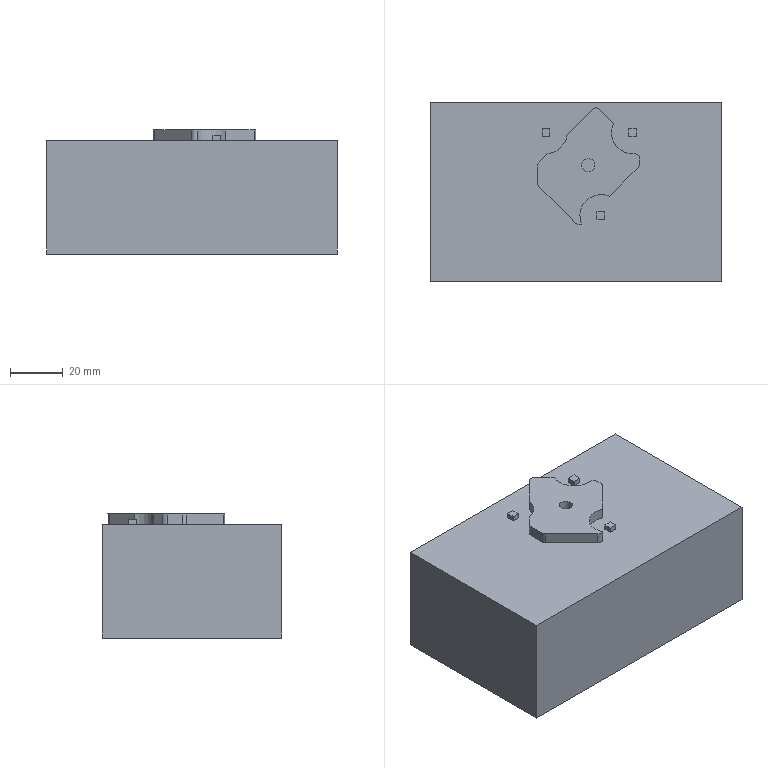NC program | NX | posted with a generic post | part box 110.151 x 68.163 x 47.1 mm
Lines 1467 to 3424 of 32691, first 1659 of 1912 lines:
(CAVITY_MILL_COPY_COPY , TOOL : D10R0)
N2902 T03 M6
N2904 G54
N2906 G17 G0 G90 X-8.338 Y22.938 S5000 M3
N2908 G43 Z80.5 H3
N2910 G94 G1 Z-34. F3000.
N2912 Z-34.5 F1500.
N2914 G3 X-11.214 Y22.865 R188.379
N2916 G1 X-11.344 Y22.861
N2918 G2 X-12.979 Y21.269 R5.579
N2920 G1 X-18.467 Y17.785
N2922 G0 Z-33.8
N2924 X-11.454 Y20.4
N2926 G1 Z-35. F3000.
N2928 X-17.954 F1500.
N2930 X-19.213
N2932 G2 X-20.334 Y20.061 R5.398
N2934 G1 X-26.723 Y18.865
N2936 G0 Z-34.3
N2938 X-11.355 Y20.4
N2940 G1 Z-35.5 F3000.
N2942 X-17.855 F1500.
N2944 X-19.184
N2946 G2 X-20.336 Y20.019 R5.5
N2948 G1 X-26.695 Y18.673
N2950 G0 Z-34.8
N2952 X-11.355 Y20.4
N2954 G1 Z-36. F3000.
N2956 X-17.855 F1500.
N2958 X-19.184
N2960 G2 X-20.336 Y20.019 R5.5
N2962 G1 X-26.695 Y18.673
N2964 G0 Z-35.3
N2966 X-11.355 Y20.4
N2968 G1 Z-36.5 F3000.
N2970 X-17.855 F1500.
N2972 X-19.184
N2974 G2 X-20.336 Y20.019 R5.5
N2976 G1 X-26.695 Y18.673
N2978 G0 Z-35.8
N2980 X-11.355 Y20.4
N2982 G1 Z-37. F3000.
N2984 X-17.855 F1500.
N2986 X-19.184
N2988 G2 X-20.336 Y20.019 R5.5
N2990 G1 X-26.695 Y18.673
N2992 G0 Z80.5
N2994 X-7.629 Y22.95
N2996 G1 Z-34.5 F3000.
N2998 Z-35. F1500.
N3000 G3 X-8.157 Y22.942 R188.379
N3002 X-10.533 Y22.886 R186.972
N3004 G1 X-10.852 Y22.663
N3006 G2 X-12.439 Y21.219 R5.626
N3008 G1 X-17.992 Y17.841
N3010 G0 Z-34.3
N3012 X-6.882 Y22.959
N3014 G1 Z-35. F3000.
N3016 Z-35.5 F1500.
N3018 G3 X-8.157 Y22.942 R188.379
N3020 X-9.727 Y22.908 R186.972
N3022 G1 X-10.131 Y22.663
N3024 X-10.533 Y22.202
N3026 G2 X-11.687 Y21.24 R5.524
N3028 G1 X-17.199 Y17.795
N3030 G0 Z-34.8
N3032 X-6.062 Y22.965
N3034 G1 Z-35.5 F3000.
N3036 Z-36. F1500.
N3038 G3 X-8.913 Y22.927 R189.402
N3040 X-9.594 Y22.347 R2.814
N3042 G2 X-10.824 Y21.273 R5.534
N3044 G1 X-16.298 Y17.769
N3046 G0 Z-35.3
N3048 X-5.086 Y22.968
N3050 G1 Z-36. F3000.
N3052 Z-36.5 F1500.
N3054 G3 X-8.103 Y22.942 R189.402
N3056 G1 X-8.735 Y22.258
N3058 G2 X-9.884 Y21.275 R5.524
N3060 G1 X-15.355 Y17.765
N3062 G0 Z-24.
N3064 X3.06 Y21.256
N3066 G1 Z-34. F3000.
N3068 Z-34.5 F1500.
N3070 G2 X1.548 Y22.663 R5.551
N3072 G1 X0.81 Y22.879
N3074 G3 X-1.65 Y22.939 R185.749
N3076 G0 Z-33.8
N3078 X2.321 Y21.298
N3080 G1 Z-34.5 F3000.
N3082 Z-35. F1500.
N3084 G2 X0.81 Y22.814 R5.053
N3086 G1 X0.018 Y22.902
N3088 G3 X-2.291 Y22.95 R185.749
N3090 G0 Z-34.3
N3092 X1.632 Y21.296
N3094 G1 Z-35. F3000.
N3096 Z-35.5 F1500.
N3098 G2 X0.001 Y22.902 R5.616
N3100 G3 X-2.481 Y22.952 R185.749
N3102 X-3.083 Y22.959 R188.379
N3104 G0 Z-34.8
N3106 X0.859 Y21.287
N3108 G1 Z-35.5 F3000.
N3110 Z-36. F1500.
N3112 G2 X-0.81 Y22.922 R5.664
N3114 G1 X-0.842 Y22.923
N3116 G3 X-3.966 Y22.965 R189.402
N3118 G0 Z-35.3
N3120 X0.008 Y21.244
N3122 G1 Z-36. F3000.
N3124 Z-36.5 F1500.
N3126 G2 X-1.621 Y22.786 R5.593
N3128 G1 X-2.431 Y22.95
N3130 G3 X-2.965 Y22.957 R181.014
N3132 X-4.972 Y22.968 R189.402
N3134 G0 Z-35.8
N3136 X-0.703 Y21.038
N3138 G1 Z-36.5 F3000.
N3140 Z-37. F1500.
N3142 G2 X-2.675 Y22.798 R5.501
N3144 G1 X-3.241 Y22.958
N3146 X-5.645 Y22.967
N3148 X-6.453 Y22.962
N3150 G3 X-7.284 Y22.798 R3.242
N3152 G2 X-9.436 Y20.953 R5.551
N3154 G1 X-15.288 Y18.124
N3156 G0 Z-36.3
N3158 X-6.996 Y13.445
N3160 G1 Z-37.5 F3000.
N3162 X-9.264 Y19.536 F1500.
N3164 X-9.266
N3166 G3 X-13.489 Y14.163 R6.56
N3168 G2 X-14.475 Y13.281 R1.
N3170 G1 Y14.
N3172 G3 X-19.975 Y19.5 R5.5
N3174 G1 X-22.975
N3176 G3 X-28.418 Y14.787 R5.5
N3178 G2 X-29.177 Y15.891 R1.
N3180 G3 X-30.443 Y20.701 R6.56
N3182 G2 X-30.326 Y22.035 R1.
N3184 G3 X-25.975 Y19.9 R5.5
N3186 G1 X-21.475
N3188 G3 X-19.184 Y20.4 R5.5
N3190 G1 X-10.468
N3192 G3 X-8.644 Y20.723 R5.611
N3194 G2 X-9.264 Y19.536 R1.
N3196 G1 X-7.004 Y13.442
N3198 G0 Z-24.
N3200 X-1.466 Y20.78
N3202 G1 Z-37. F3000.
N3204 Z-37.5 F1500.
N3206 G2 X-2.059 Y21.044 R5.797
N3208 X-4.051 Y22.85 R5.402
N3210 G3 X-4.795 Y22.964 R5.482
N3212 G1 X-5.672 Y22.967
N3214 X-5.926 Y22.798
N3216 X-6.121 Y22.528
N3218 G2 X-8.543 Y20.76 R5.611
N3220 G1 X-14.626 Y18.469
N3222 G0 Z-36.8
N3224 X-6.995 Y13.075
N3226 G1 Z-38. F3000.
N3228 X-9.149 Y19.208 F1500.
N3230 G3 X-13.483 Y13.843 R6.56
N3232 G2 X-14.475 Y12.969 R1.
N3234 G1 Y14.
N3236 G3 X-19.975 Y19.5 R5.5
N3238 G1 X-22.975
N3240 G3 X-28.418 Y14.787 R5.5
N3242 G2 X-29.177 Y15.891 R1.
N3244 G3 X-30.443 Y20.701 R6.56
N3246 G2 X-30.326 Y22.035 R1.
N3248 G3 X-25.975 Y19.9 R5.5
N3250 G1 X-21.475
N3252 G3 X-19.184 Y20.4 R5.5
N3254 G1 X-8.783
N3256 X-8.788 Y20.326
N3258 X-8.703 Y20.316
N3260 X-8.691 Y20.389
N3262 G3 X-7.659 Y20.495 R5.482
N3264 G2 X-8.504 Y19.399 R1.002
N3266 G1 X-8.544 Y19.388
N3268 G3 X-9.149 Y19.208 R6.56
N3270 G1 X-6.995 Y13.075
N3272 G0 Z-24.
N3274 X-2.444 Y20.534
N3276 G1 Z-37.5 F3000.
N3278 Z-38. F1500.
N3280 G2 X-4.944 Y21.837 R5.502
N3282 G1 X-5.097 Y21.761
N3284 X-5.264 Y21.624
N3286 G2 X-7.494 Y20.53 R5.482
N3288 G1 X-13.826 Y19.064
N3290 G0 Z-24.
N3292 X0.082 Y14.392
N3294 G1 Z-34.5 F3000.
N3296 X5.683 Y17.69 F1500.
N3298 G3 X3.527 Y19.912 R6.56
N3300 G2 X3.16 Y21.194 R1.
N3302 G3 X5.999 Y20.4 R5.551
N3304 G1 X9.302
N3306 G3 X10.889 Y20.156 R4.677
N3308 G1 X16.023
N3310 G3 X21.082 Y23.438 R5.434
N3312 G2 X21.535 Y22.198 R1.
N3314 G3 X21.552 Y17.401 R6.56
N3316 G2 X21.093 Y16.151 R1.
N3318 G3 X16.048 Y19.5 R5.481
N3320 G1 X13.065
N3322 G3 X7.525 Y14.079 R5.481
N3324 G1 Y13.785
N3326 G2 X6.58 Y14.728 R1.
N3328 G3 X5.683 Y17.69 R6.56
N3330 G1 X0.082 Y14.392
N3332 G0 Z-33.8
N3334 X0.068 Y14.09
N3336 G1 Z-35. F3000.
N3338 X5.54 Y17.599 F1500.
N3340 G3 X3.206 Y19.79 R6.56
N3342 G2 X2.766 Y21.042 R1.
N3344 G3 X5.361 Y20.4 R5.867
N3346 G1 X9.263
N3348 G3 X11.376 Y19.969 R5.124
N3350 G1 X16.025
N3352 G3 X21.13 Y23.415 R5.494
N3354 G2 X21.605 Y22.159 R1.
N3356 G3 X21.623 Y17.302 R6.56
N3358 G2 X21.145 Y16.035 R1.
N3360 G3 X16.048 Y19.5 R5.468
N3362 G1 X13.065
N3364 G3 X7.525 Y14.079 R5.474
N3366 G1 Y13.634
N3368 G2 X6.562 Y14.55 R1.
N3370 G3 X6.522 Y14.911 R6.56
N3372 X5.54 Y17.599 R6.56
N3374 G1 X0.068 Y14.09
N3376 G0 Z-34.3
N3378 X0.074 Y13.794
N3380 G1 Z-35.5 F3000.
N3382 X5.409 Y17.508 F1500.
N3384 G3 X2.876 Y19.668 R6.56
N3386 G2 X2.366 Y20.896 R1.
N3388 G3 X4.648 Y20.4 R5.616
N3390 G1 X9.234
N3392 G3 X11.525 Y19.9 R5.5
N3394 G1 X16.025
N3396 G3 X21.128 Y23.348 R5.5
N3398 G2 X21.605 Y22.096 R1.
N3400 G3 X21.626 Y17.295 R6.56
N3402 G2 X21.147 Y16.031 R1.
N3404 G3 X16.074 Y19.5 R5.468
N3406 G1 X13.065
N3408 G3 X7.525 Y14.079 R5.467
N3410 G1 Y13.523
N3412 G2 X6.552 Y14.421 R1.
N3414 G3 X5.409 Y17.508 R6.56
N3416 G1 X0.074 Y13.794
N3418 G0 Z-34.8
N3420 X0.073 Y13.509
N3422 G1 Z-36. F3000.
N3424 X5.275 Y17.407 F1500.
N3426 G3 X2.419 Y19.58 R6.56
N3428 G2 X1.825 Y20.795 R1.
N3430 G3 X3.847 Y20.4 R5.664
N3432 G1 X9.234
N3434 G3 X11.525 Y19.9 R5.5
N3436 G1 X16.025
N3438 G3 X21.124 Y23.338 R5.5
N3440 G2 X21.598 Y22.085 R1.
N3442 G3 X21.579 Y17.364 R6.56
N3444 G2 X21.11 Y16.123 R1.
N3446 G3 X16.025 Y19.5 R5.468
N3448 G1 X13.065
N3450 G3 X7.525 Y14. R5.467
N3452 G1 Y13.352
N3454 G2 X6.541 Y14.235 R1.
N3456 G3 X5.275 Y17.407 R6.56
N3458 G1 X0.073 Y13.509
N3460 G0 Z-35.3
N3462 X0.072 Y13.262
N3464 G1 Z-36.5 F3000.
N3466 X5.156 Y17.312 F1500.
N3468 G3 X1.975 Y19.488 R6.56
N3470 G2 X1.295 Y20.654 R1.
N3472 G3 X2.91 Y20.4 R5.593
N3474 G1 X9.234
N3476 G3 X11.525 Y19.9 R5.5
N3478 G1 X16.025
N3480 G3 X21.124 Y23.338 R5.5
N3482 G2 X21.598 Y22.085 R1.
N3484 G3 X21.579 Y17.364 R6.56
N3486 G2 X21.11 Y16.123 R1.
N3488 G3 X16.025 Y19.5 R5.468
N3490 G1 X13.065
N3492 G3 X7.525 Y14. R5.467
N3494 G1 Y13.166
N3496 G2 X6.534 Y14.041 R1.
N3498 G3 X5.156 Y17.312 R6.56
N3500 G1 X0.072 Y13.262
N3502 G0 Z-35.8
N3504 X0.071 Y13.054
N3506 G1 Z-37. F3000.
N3508 X5.054 Y17.227 F1500.
N3510 G3 X1.408 Y19.428 R6.56
N3512 G2 X0.628 Y20.541 R1.
N3514 G3 X1.875 Y20.4 R5.501
N3516 G1 X9.234
N3518 G3 X11.525 Y19.9 R5.5
N3520 G1 X16.025
N3522 G3 X21.124 Y23.338 R5.5
N3524 G2 X21.598 Y22.085 R1.
N3526 G3 X21.579 Y17.364 R6.56
N3528 G2 X21.11 Y16.123 R1.
N3530 G3 X16.025 Y19.5 R5.468
N3532 G1 X13.065
N3534 G3 X7.525 Y14. R5.467
N3536 G1 Y12.966
N3538 G2 X6.533 Y13.84 R1.
N3540 G3 X5.054 Y17.227 R6.56
N3542 G1 X0.071 Y13.054
N3544 G0 Z-36.3
N3546 X5.412 Y16.995
N3548 G1 Z-37. F3000.
N3550 Z-37.5 F1500.
N3552 G3 X4.525 Y14. R5.5
N3554 G1 Y13.293
N3556 G2 X3.54 Y14.176 R1.
N3558 G3 X-0.624 Y19.531 R6.56
N3560 G2 X-1.238 Y20.698 R1.
N3562 G3 X0.524 Y20.4 R5.797
N3564 G1 X9.234
N3566 G3 X11.525 Y19.9 R5.5
N3568 G1 X16.025
N3570 G3 X21.124 Y23.338 R5.5
N3572 G2 X21.598 Y22.085 R1.
N3574 G3 X21.579 Y17.364 R6.56
N3576 G2 X21.11 Y16.123 R1.
N3578 G3 X16.025 Y19.5 R5.468
N3580 G1 X13.065
N3582 X12.918
N3584 X10.025
N3586 G3 X5.412 Y16.995 R5.5
N3588 G0 Z-36.8
N3590 G1 Z-37.5 F3000.
N3592 Z-38. F1500.
N3594 G3 X4.525 Y14. R5.5
N3596 G1 Y12.969
N3598 G2 X3.533 Y13.844 R1.
N3600 G3 X-1.561 Y19.425 R6.56
N3602 G2 X-2.339 Y20.512 R1.
N3604 G3 X-1.24 Y20.4 R5.502
N3606 G1 X9.234
N3608 G3 X11.525 Y19.9 R5.5
N3610 G1 X16.025
N3612 G3 X21.124 Y23.338 R5.5
N3614 G2 X21.598 Y22.085 R1.
N3616 G3 X21.579 Y17.364 R6.56
N3618 G2 X21.11 Y16.123 R1.
N3620 G3 X16.025 Y19.5 R5.468
N3622 G1 X10.025
N3624 G3 X5.412 Y16.995 R5.5
N3626 G0 Z80.5
(CAVITY_MILL , TOOL : D10R0)
N3628 X11.108 Y-48.641
N3630 Z80.
N3632 G1 Z-38. F3000.
N3634 Y-42.141 F1500.
N3636 X-39.278
N3638 X-39.321 Y-42.124
N3640 X-53.118 Y-28.327
N3642 X-53.135 Y-28.284
N3644 Y24.042
N3646 X-53.118 Y24.084
N3648 X-35.078 Y42.124
N3650 X-35.036 Y42.141
N3652 X29.328
N3654 X29.371 Y42.124
N3656 X53.118 Y18.377
N3658 X53.135 Y18.335
N3660 Y-14.092
N3662 X53.118 Y-14.134
N3664 X25.128 Y-42.124
N3666 X25.086 Y-42.141
N3668 X11.108
N3670 Y-34.641
N3672 X-36.196
N3674 X-45.635 Y-25.203
N3676 Y20.96
N3678 X-32.871 Y33.724
N3680 G3 X-32.875 Y33.5 R6.9
N3682 G1 Y25.4
N3684 G3 X-27.944 Y18.787 R6.9
N3686 X-29.875 Y14. R6.9
N3688 G1 Y11.
N3690 G3 X-22.975 Y4.1 R6.9
N3692 G1 X-19.975
N3694 G3 X-13.075 Y11. R6.9
N3696 G1 Y14.
N3698 G3 X-15.22 Y19. R6.9
N3700 G1 X-16.254 Y17.913
N3702 G2 X-14.575 Y14. R5.4
N3704 G1 Y11.
N3706 G2 X-19.975 Y5.6 R5.4
N3708 G1 X-22.975
N3710 G2 X-28.375 Y11. R5.4
N3712 G1 Y14.
N3714 G2 X-22.975 Y19.4 R5.4
N3716 G1 X-19.975
N3718 G2 X-16.254 Y17.913 R5.4
N3720 G1 X-15.22 Y19.
N3722 X-8.709
N3724 G3 X-4.975 Y20.099 R6.915
N3726 X-1.201 Y19. R6.91
N3728 G1 X5.27
N3730 G3 X3.125 Y14. R6.9
N3732 G1 Y11.
N3734 G3 X10.025 Y4.1 R6.9
N3736 G1 X16.025
N3738 G3 X22.925 Y11. R6.9
N3740 G1 Y14.
N3742 G3 X19.914 Y19.7 R6.9
N3744 G1 X19.068 Y18.461
N3746 G2 X21.425 Y14. R5.4
N3748 G1 Y11.
N3750 G2 X16.025 Y5.6 R5.4
N3752 G1 X10.025
N3754 G2 X4.625 Y11. R5.4
N3756 G1 Y14.
N3758 G2 X10.025 Y19.4 R5.4
N3760 G1 X16.025
N3762 G2 X19.068 Y18.461 R5.4
N3764 G1 X19.914 Y19.7
N3766 G3 X22.925 Y25.4 R6.9
N3768 G1 Y33.5
N3770 G3 X22.83 Y34.641 R6.9
N3772 G1 X21.351 Y34.393
N3774 G2 X21.425 Y33.5 R5.4
N3776 G1 Y25.4
N3778 G2 X16.025 Y20. R5.4
N3780 G1 X11.525
N3782 G2 X9.349 Y20.458 R5.4
N3784 G1 X9.259 Y20.5
N3786 X-1.205
N3788 G2 X-4.556 Y21.638 R5.41
N3790 G1 X-5.224 Y21.776
N3792 G2 X-8.709 Y20.5 R5.415
N3794 G1 X-19.206
N3796 G2 X-21.475 Y20. R5.4
N3798 G1 X-25.975
N3800 G2 X-31.375 Y25.4 R5.4
N3802 G1 Y33.5
N3804 G2 X-29.793 Y37.318 R5.4
N3806 G1 X-28.793 Y38.318
N3808 G2 X-24.975 Y39.9 R5.4
N3810 G1 X15.025
N3812 G2 X18.844 Y38.318 R5.4
N3814 G1 X19.844 Y37.318
N3816 G2 X21.351 Y34.393 R5.4
N3818 G1 X22.83 Y34.641
N3820 X26.247
N3822 X45.635 Y15.253
N3824 Y-11.01
N3826 X22.004 Y-34.641
N3828 X11.108
N3830 Y-27.141
N3832 X-6.104
N3834 G3 X-1.075 Y-20.5 R6.9
N3836 G1 Y-17.5
N3838 G3 X-7.975 Y-10.6 R6.9
N3840 G1 X-10.975
N3842 G3 X-17.875 Y-17.5 R6.9
N3844 G1 Y-20.5
N3846 G3 X-12.846 Y-27.141 R6.9
N3848 G1 X-12.439 Y-25.698
N3850 G2 X-16.375 Y-20.5 R5.4
N3852 G1 Y-17.5
N3854 G2 X-10.975 Y-12.1 R5.4
N3856 G1 X-7.975
N3858 G2 X-2.575 Y-17.5 R5.4
N3860 G1 Y-20.5
N3862 G2 X-7.975 Y-25.9 R5.4
N3864 G1 X-10.975
N3866 G2 X-12.439 Y-25.698 R5.4
N3868 G1 X-12.846 Y-27.141
N3870 X-33.09
N3872 X-38.135 Y-22.096
N3874 Y17.688
N3876 G3 X-37.181 Y16.356 R14.4
N3878 X-37.375 Y14. R14.4
N3880 G1 Y11.
N3882 G3 X-23.495 Y-3.391 R14.4
N3884 G1 X-23.766 Y-10.886
N3886 G3 X-25.375 Y-17.5 R14.4
N3888 G1 Y-19.641
N3890 X-29.983
N3892 X-30.635 Y-18.989
N3894 Y-9.516
N3896 G3 X-23.766 Y-10.886 R21.9
N3898 G1 X-19.067 Y-8.542
N3900 X-23.766 Y-10.886
N3902 X-23.495 Y-3.391
N3904 G3 X-22.975 Y-3.4 R14.4
N3906 G1 X-19.975
N3908 G3 X-5.575 Y11. R14.4
N3910 G1 Y11.846
N3912 G3 X-4.975 Y11.993 R14.415
N3914 X-4.375 Y11.846 R14.41
N3916 G1 Y11.
N3918 G3 X10.025 Y-3.4 R14.4
N3920 G1 X16.025
N3922 G3 X30.425 Y11. R14.4
N3924 G1 Y14.
N3926 G3 X29.249 Y19.7 R14.4
N3928 X29.622 Y20.659 R14.4
N3930 G1 X28.059 Y25.583
N3932 X29.622 Y20.659
N3934 X38.135 Y12.146
N3936 Y-7.904
N3938 X18.897 Y-27.141
N3940 X11.108
N3942 Y-19.641
N3944 X6.425
N3946 Y-17.5
N3948 G3 X4.42 Y-10.171 R14.4
N3950 G1 X1.252 Y-6.303
N3952 G2 X-4.975 Y-1.303 R19.4
N3954 X-9.935 Y-5.6 R19.4
N3956 G1 X-7.975
N3958 G2 X-0.268 Y-8.433 R11.9
N3960 X1.252 Y-6.303 R5.
N3962 G1 X4.42 Y-10.171
N3964 G3 X10.025 Y-10.9 R21.9
N3966 G1 X16.025
N3968 G3 X28.287 Y-7.146 R21.9
N3970 G1 X32.189 Y-1.945
N3972 X28.287 Y-7.146
N3974 X15.791 Y-19.641
N3976 X11.108
N3978 Y-26.141
N3980 G0 Z80.
(CAVITY_MILL_1 , TOOL : D10R0)
N3982 X-5.489 Y-3.273 S4000
N3984 G1 Z-37. F5000.
N3986 X-5.018 Y-3.457 Z-37.044 F1500.
N3988 X-3.609 Y-4.247 Z-37.186
N3990 X-2.32 Y-5.221 Z-37.327
N3992 X-1.192 Y-6.349 Z-37.466
N3994 X1.103 Y-4.054 Z-37.75
N3996 X1.193 Y-3.976 Z-37.761
N3998 X1.875 Y-3.476 Z-37.835
N4000 X-2.841 Y1.24 Z-38.418
N4002 X-7.556 Y5.955
N4004 X-10.526 Y2.985
N4006 X-8.793 Y1.253
N4008 G2 X-6.124 Y-2.831 R11.9
N4010 G1 X-5.806 Y-3.149
N4012 G2 X-1.722 Y-5.818 R11.9
N4014 G1 X-1.192 Y-6.349
N4016 X0.505 Y-4.652
N4018 G2 X1.875 Y-3.476 R11.9
N4020 G1 X-2.841 Y1.24
N4022 X1.756 Y5.836
N4024 X-7.556 Y15.147
N4026 X-18.773 Y3.93
N4028 Y0.913
N4030 X-18.671 Y0.891
N4032 G2 X-16.218 Y-0.515 R5.4
N4034 G1 X-13.389 Y-3.344
N4036 G2 X-11.916 Y-6.087 R5.4
N4038 G1 X-11.888 Y-6.259
N4040 X-9.234 Y-8.913
N4042 X-9.094 Y-8.94
N4044 X-9.063 Y-8.941
N4046 G2 X-6.318 Y-10.415 R5.4
N4048 G1 X-3.49 Y-13.243
N4050 G2 X-1.983 Y-16.164 R5.4
N4052 G1 X-1.192 Y-16.955
N4054 X0.771 Y-14.992
N4056 X0.803 Y-14.825
N4058 X0.806 Y-14.789
N4060 G2 X2.273 Y-12.076 R5.4
N4062 G1 X5.101 Y-9.248
N4064 G2 X8.022 Y-7.741 R5.4
N4066 G1 X9.318 Y-6.445
N4068 Y-1.727
N4070 X1.756 Y5.836
N4072 X-1.78 Y2.3
N4074 G0 Z-37.4
N4076 X-5.489 Y-3.273
N4078 G1 Z-37.918 F5000.
N4080 X-5.018 Y-3.457 Z-37.962 F1500.
N4082 X-3.609 Y-4.247 Z-38.104
N4084 X-2.32 Y-5.221 Z-38.245
N4086 X-1.192 Y-6.349 Z-38.385
N4088 X1.103 Y-4.054 Z-38.669
N4090 X1.193 Y-3.976 Z-38.679
N4092 X1.875 Y-3.476 Z-38.753
N4094 X-2.841 Y1.24 Z-39.336
N4096 X-7.556 Y5.955
N4098 X-10.526 Y2.985
N4100 X-8.793 Y1.253
N4102 G2 X-6.124 Y-2.831 R11.9
N4104 G1 X-5.806 Y-3.149
N4106 G2 X-1.722 Y-5.818 R11.9
N4108 G1 X-1.192 Y-6.349
N4110 X0.505 Y-4.652
N4112 G2 X1.875 Y-3.476 R11.9
N4114 G1 X-2.841 Y1.24
N4116 X1.756 Y5.836
N4118 X-7.556 Y15.147
N4120 X-18.773 Y3.93
N4122 Y0.915
N4124 X-18.671 Y0.891
N4126 G2 X-16.218 Y-0.515 R5.4
N4128 G1 X-13.389 Y-3.344
N4130 G2 X-11.916 Y-6.087 R5.4
N4132 G1 X-11.886 Y-6.262
N4134 X-9.236 Y-8.911
N4136 X-9.093 Y-8.938
N4138 X-9.063 Y-8.941
N4140 G2 X-6.318 Y-10.415 R5.4
N4142 G1 X-3.49 Y-13.243
N4144 G2 X-1.983 Y-16.164 R5.4
N4146 G1 X-1.192 Y-16.955
N4148 X0.769 Y-14.995
N4150 X0.806 Y-14.789
N4152 G2 X2.273 Y-12.076 R5.4
N4154 G1 X5.101 Y-9.248
N4156 G2 X8.022 Y-7.741 R5.4
N4158 G1 X9.318 Y-6.445
N4160 Y-1.727
N4162 X1.756 Y5.836
N4164 X-1.78 Y2.3
N4166 G0 Z-38.318
N4168 X-5.489 Y-3.273
N4170 G1 Z-38.836 F5000.
N4172 X-5.018 Y-3.457 Z-38.881 F1500.
N4174 X-3.609 Y-4.247 Z-39.022
N4176 X-2.32 Y-5.221 Z-39.163
N4178 X-1.192 Y-6.349 Z-39.303
N4180 X1.103 Y-4.054 Z-39.587
N4182 X1.193 Y-3.976 Z-39.597
N4184 X1.875 Y-3.476 Z-39.671
N4186 X-2.841 Y1.24 Z-40.255
N4188 X-7.556 Y5.955
N4190 X-10.526 Y2.985
N4192 X-8.793 Y1.253
N4194 G2 X-6.124 Y-2.831 R11.9
N4196 G1 X-5.806 Y-3.149
N4198 G2 X-1.722 Y-5.818 R11.9
N4200 G1 X-1.192 Y-6.349
N4202 X0.505 Y-4.652
N4204 G2 X1.875 Y-3.476 R11.9
N4206 G1 X-2.841 Y1.24
N4208 X1.756 Y5.836
N4210 X-7.556 Y15.147
N4212 X-18.773 Y3.93
N4214 Y0.916
N4216 X-18.671 Y0.891
N4218 G2 X-16.218 Y-0.515 R5.4
N4220 G1 X-13.389 Y-3.344
N4222 G2 X-11.916 Y-6.087 R5.4
N4224 G1 X-11.883 Y-6.264
N4226 X-9.238 Y-8.909
N4228 X-9.063 Y-8.941
N4230 G2 X-6.318 Y-10.415 R5.4
N4232 G1 X-3.49 Y-13.243
N4234 G2 X-1.983 Y-16.164 R5.4
N4236 G1 X-1.192 Y-16.955
N4238 X0.766 Y-14.997
N4240 G2 X2.273 Y-12.076 R5.4
N4242 G1 X5.101 Y-9.248
N4244 G2 X8.022 Y-7.741 R5.4
N4246 G1 X9.318 Y-6.445
N4248 Y-1.727
N4250 X1.756 Y5.836
N4252 X-1.78 Y2.3
N4254 G0 Z-39.236
N4256 X-7.224 Y2.507
N4258 G1 Z-39.755 F5000.
N4260 X-7.983 Y1.748 Z-39.848 F1500.
N4262 X-1.722 Y-4.513 Z-40.623
N4264 X-0.411 Y-3.202 Z-40.785
N4266 X-3.541 Y-0.072 Z-41.173
N4268 X-6.672 Y3.059
N4270 X-7.983 Y1.748
N4272 X-1.722 Y-4.513
N4274 X-0.411 Y-3.202
N4276 X-3.541 Y-0.072
N4278 X1.055 Y4.525
N4280 X-6.672 Y12.251
N4282 X-17.176 Y1.748
N4284 X-1.722 Y-13.706
N4286 X8.304 Y-3.679
N4288 Y-2.725
N4290 X1.055 Y4.525
N4292 X-2.481 Y0.989
N4294 G0 Z-40.155
N4296 X-4.027 Y-1.392
N4298 G1 Z-40.673 F5000.
N4300 X-1.722 Y-3.697 Z-40.958 F1500.
N4302 X-1.227 Y-3.202 Z-41.019
N4304 X-6.672 Y2.243 Z-41.693
N4306 X-7.167 Y1.748 Z-41.754
N4308 X-4.445 Y-0.975 Z-42.091
N4310 X-1.722 Y-3.697
N4312 X-1.227 Y-3.202
N4314 X-6.672 Y2.243
N4316 X-7.167 Y1.748
N4318 X-4.445 Y-0.975
N4320 X-9.041 Y-5.571
N4322 X-1.722 Y-12.889
N4324 X7.727 Y-3.44
N4326 Y-2.964
N4328 X-6.672 Y11.435
N4330 X-16.359 Y1.748
N4332 X-9.041 Y-5.571
N4334 X-5.505 Y-2.035
N4336 G0 Z-41.073
N4338 X-4.027 Y-1.392
N4340 G1 Z-41.591 F5000.
N4342 X-1.722 Y-3.697 Z-41.876 F1500.
N4344 X-1.227 Y-3.202 Z-41.937
N4346 X-6.672 Y2.243 Z-42.611
N4348 X-7.167 Y1.748 Z-42.672
N4350 X-4.445 Y-0.975 Z-43.009
N4352 X-1.722 Y-3.697
N4354 X-1.227 Y-3.202
N4356 X-6.672 Y2.243
N4358 X-7.167 Y1.748
N4360 X-4.445 Y-0.975
N4362 X-9.041 Y-5.571
N4364 X-1.722 Y-12.889
N4366 X7.727 Y-3.44
N4368 Y-2.964
N4370 X-6.672 Y11.435
N4372 X-16.359 Y1.748
N4374 X-9.041 Y-5.571
N4376 X-5.505 Y-2.035
N4378 G0 Z-41.991
N4380 X-4.027 Y-1.392
N4382 G1 Z-42.509 F5000.
N4384 X-1.722 Y-3.697 Z-42.794 F1500.
N4386 X-1.227 Y-3.202 Z-42.856
N4388 X-6.672 Y2.243 Z-43.529
N4390 X-7.167 Y1.748 Z-43.59
N4392 X-4.445 Y-0.975 Z-43.927
N4394 X-1.722 Y-3.697
N4396 X-1.227 Y-3.202
N4398 X-6.672 Y2.243
N4400 X-7.167 Y1.748
N4402 X-4.445 Y-0.975
N4404 X-9.041 Y-5.571
N4406 X-1.722 Y-12.889
N4408 X7.727 Y-3.44
N4410 Y-2.964
N4412 X-6.672 Y11.435
N4414 X-16.359 Y1.748
N4416 X-9.041 Y-5.571
N4418 X-5.505 Y-2.035
N4420 G0 Z-42.909
N4422 X-4.027 Y-1.392
N4424 G1 Z-43.427 F5000.
N4426 X-1.722 Y-3.697 Z-43.712 F1500.
N4428 X-1.227 Y-3.202 Z-43.774
N4430 X-6.672 Y2.243 Z-44.447
N4432 X-7.167 Y1.748 Z-44.509
N4434 X-4.445 Y-0.975 Z-44.845
N4436 X-1.722 Y-3.697
N4438 X-1.227 Y-3.202
N4440 X-6.672 Y2.243
N4442 X-7.167 Y1.748
N4444 X-4.445 Y-0.975
N4446 X-9.041 Y-5.571
N4448 X-1.722 Y-12.889
N4450 X7.727 Y-3.44
N4452 Y-2.964
N4454 X-6.672 Y11.435
N4456 X-16.359 Y1.748
N4458 X-9.041 Y-5.571
N4460 X-5.505 Y-2.035
N4462 G0 Z-43.827
N4464 X-4.027 Y-1.392
N4466 G1 Z-44.345 F5000.
N4468 X-1.722 Y-3.697 Z-44.631 F1500.
N4470 X-1.227 Y-3.202 Z-44.692
N4472 X-6.672 Y2.243 Z-45.366
N4474 X-7.167 Y1.748 Z-45.427
N4476 X-4.445 Y-0.975 Z-45.764
N4478 X-1.722 Y-3.697
N4480 X-1.227 Y-3.202
N4482 X-6.672 Y2.243
N4484 X-7.167 Y1.748
N4486 X-4.445 Y-0.975
N4488 X-9.041 Y-5.571
N4490 X-1.722 Y-12.889
N4492 X7.727 Y-3.44
N4494 Y-2.964
N4496 X-6.672 Y11.435
N4498 X-16.359 Y1.748
N4500 X-9.041 Y-5.571
N4502 X-5.505 Y-2.035
N4504 G0 Z-44.745
N4506 X-4.027 Y-1.392
N4508 G1 Z-45.264 F5000.
N4510 X-1.722 Y-3.697 Z-45.549 F1500.
N4512 X-1.227 Y-3.202 Z-45.61
N4514 X-6.672 Y2.243 Z-46.284
N4516 X-7.167 Y1.748 Z-46.345
N4518 X-4.445 Y-0.975 Z-46.682
N4520 X-1.722 Y-3.697
N4522 X-1.227 Y-3.202
N4524 X-6.672 Y2.243
N4526 X-7.167 Y1.748
N4528 X-4.445 Y-0.975
N4530 X-9.041 Y-5.571
N4532 X-1.722 Y-12.889
N4534 X7.727 Y-3.44
N4536 Y-2.964
N4538 X-6.672 Y11.435
N4540 X-16.359 Y1.748
N4542 X-9.041 Y-5.571
N4544 X-5.505 Y-2.035
N4546 G0 Z-45.664
N4548 X-4.027 Y-1.392
N4550 G1 Z-46.182 F5000.
N4552 X-1.722 Y-3.697 Z-46.467 F1500.
N4554 X-1.227 Y-3.202 Z-46.528
N4556 X-6.672 Y2.243 Z-47.202
N4558 X-7.167 Y1.748 Z-47.263
N4560 X-4.445 Y-0.975 Z-47.6
N4562 X-1.722 Y-3.697
N4564 X-1.227 Y-3.202
N4566 X-6.672 Y2.243
N4568 X-7.167 Y1.748
N4570 X-4.445 Y-0.975
N4572 X-9.041 Y-5.571
N4574 X-1.722 Y-12.889
N4576 X7.727 Y-3.44
N4578 Y-2.964
N4580 X-6.672 Y11.435
N4582 X-16.359 Y1.748
N4584 X-9.041 Y-5.571
N4586 X-5.505 Y-2.035
N4588 G0 Z80.
N4590 M5
(DRILLING , TOOL : DK-Ø8)
N4592 T04 M6
N4594 G54
N4596 G17 G0 G90 X-49.411 Y19.207 S2000 M3
N4598 G43 Z22. H4
N4600 G94 G81 G99 Z-40.5 F200. R-36.5
N4602 G0 Z22.
N4604 G81 X21.011 Y-38.237 Z-40.5 R-36.5
N4606 G0 Z22.
N4608 G81 X27.482 Y36.677 Z-40.5 R-36.5
N4610 G0 Z22.
N4612 G80
N4614 G0 X27.482 Y36.677 Z22.
(DRILLING_COPY , TOOL : DK-Ø8)
N4616 X26.025 Y14.5
N4618 G81 Z-39.5 F200. R-36.5
N4620 G0 Z22.
N4622 G81 Y-18.5 Z-39.5 R-36.5
N4624 G0 Z22.
N4626 G81 X-41.475 Y-12. Z-39.5 R-36.5
N4628 G0 Z22.
N4630 G81 X-39.975 Y13. Z-39.5 R-36.5
N4632 G0 Z22.
N4634 G80
N4636 G0 X-39.975 Y13. Z22.
(DRILLING_COPY_COPY , TOOL : DK-Ø8)
N4638 X-46.694 Y11.435
N4640 G81 Z-39.85 F200. R-36.5
N4642 G0 Z22.
N4644 G81 X43.462 Y2.596 Z-39.85 R-36.5
N4646 G0 Z22.
N4648 G80
N4650 G0 X43.462 Y2.596 Z22.
(DRILLING_COPY_COPY_COPY , TOOL : DK-Ø8)
N4652 X18.025 Y3.
N4654 G81 Z-39.35 F200. R-36.5
N4656 G0 Z22.
N4658 G81 Y-11. Z-39.35 R-36.5
N4660 G0 Z22.
N4662 G81 X-27.975 Z-39.35 R-36.5
N4664 G0 Z22.
N4666 G81 Y3. Z-39.35 R-36.5
N4668 G0 Z22.
N4670 G80
N4672 G0 X-27.975 Y3. Z22.
(PLANAR_MILL_COPY , TOOL : DK-Ø8)
N4674 Z42. S3500
N4676 X-7.096 Y-46.181
N4678 G1 Z-39.5 F5000.
N4680 G41 Y-43.781 F1200. D4
N4682 X-39.278
N4684 G2 X-40.48 Y-43.284 R1.7
N4686 G1 X-54.277 Y-29.486
N4688 G2 X-54.775 Y-28.284 R1.7
N4690 G1 Y24.042
N4692 G2 X-54.277 Y25.244 R1.7
N4694 G1 X-36.238 Y43.284
N4696 G2 X-35.036 Y43.781 R1.7
N4698 G1 X29.328
N4700 G2 X30.531 Y43.284 R1.7
N4702 G1 X54.277 Y19.537
N4704 G2 X54.775 Y18.335 R1.7
N4706 G1 Y-14.092
N4708 G2 X54.277 Y-15.294 R1.7
N4710 G1 X26.288 Y-43.284
N4712 G2 X25.086 Y-43.781 R1.7
N4714 G1 X-7.096
N4716 G40
N4718 Y-46.181
N4720 G0 Z42.
N4722 M5
(DRILLING_COPY_COPY_COPY_COPY , TOOL : D1.8钻头)
N4724 T05 M6
N4726 G54
N4728 G17 G0 G90 X18.025 Y3. S1800 M3
N4730 G43 Z22. H5
N4732 G94 G81 G99 Z-41.5 F100. R-36.5
N4734 G0 Z22.
N4736 G81 Y-11. Z-41.5 R-36.5
N4738 G0 Z22.
N4740 G81 X-27.975 Z-41.5 R-36.5
N4742 G0 Z22.
N4744 G81 Y3. Z-41.5 R-36.5
N4746 G0 Z22.
N4748 G80
N4750 G0 X-27.975 Y3. Z22.
N4752 M5
(DRILLING_COPY_COPY_COPY_1 , TOOL : D2.75钻头)
N4754 T06 M6
N4756 G54
N4758 G17 G0 G90 X-46.694 Y11.435 S2000 M3
N4760 G43 Z22. H6
N4762 G94 G81 G99 Z-48. F100. R-36.5
N4764 G0 Z22.
N4766 G81 X43.462 Y2.596 Z-48. R-36.5
N4768 G0 Z22.
N4770 G80
N4772 G0 X43.462 Y2.596 Z22.
N4774 M5
(PLANAR_MILL_COPY_1 , TOOL : D10R0)
N4776 T09 M6
N4778 G54
N4780 G17 G0 G90 X60.456 Y-17.149 S4000 M3
N4782 G43 Z44.75 H9
N4784 G94 G1 Z-48.4 F5000.
N4786 X57.685 Y-16.001 F800.
N4788 G2 X56.601 Y-17.623 R5.
N4790 G1 X28.617 Y-45.607
N4792 G2 X25.082 Y-47.071 R5.
N4794 G1 X-39.274
N4796 G2 X-42.81 Y-45.607 R5.
N4798 G1 X-56.601 Y-31.816
N4800 G2 X-58.065 Y-28.28 R5.
N4802 G1 Y24.037
N4804 G2 X-56.601 Y27.573 R5.
N4806 G1 X-38.567 Y45.607
N4808 G2 X-35.031 Y47.071 R5.
N4810 G1 X29.324
N4812 G2 X32.86 Y45.607 R5.
N4814 G1 X56.601 Y21.866
N4816 G2 X58.065 Y18.33 R5.
N4818 G1 Y-14.088
N4820 G2 X57.685 Y-16.001 R5.
N4822 G1 X60.456 Y-17.149
N4824 G0 Z44.75
N4826 M5
(FACE_MILLING_COPY , TOOL : E63)
N4828 T01 M6
N4830 G54
N4832 G17 G0 G90 X90.875 Y-24.527 S3500 M3
N4834 G43 Z88. H1
N4836 G94 G1 Z7.1 F5000.
N4838 X84.575 F2500.
N4840 X-84.575
N4842 Y24.527
N4844 X84.575
N4846 X90.875
N4848 G0 Y-24.527 Z6.2
N4850 G1 X84.575
N4852 X-84.575
N4854 Y24.527
N4856 X84.575
N4858 X90.875
N4860 G0 Y-24.527 Z5.3
N4862 G1 X84.575
N4864 X-84.575
N4866 Y24.527
N4868 X84.575
N4870 X90.875
N4872 G0 Y-24.527 Z4.4
N4874 G1 X84.575
N4876 X-84.575
N4878 Y24.527
N4880 X84.575
N4882 X90.875
N4884 G0 Y-24.527 Z3.5
N4886 G1 X84.575
N4888 X-84.575
N4890 Y24.527
N4892 X84.575
N4894 X90.875
N4896 G0 Y-24.527 Z2.6
N4898 G1 X84.575
N4900 X-84.575
N4902 Y24.527
N4904 X84.575
N4906 X90.875
N4908 G0 Y-24.527 Z1.7
N4910 G1 X84.575
N4912 X-84.575
N4914 Y24.527
N4916 X84.575
N4918 X90.875
N4920 G0 Y-24.527 Z0.8
N4922 G1 X84.575
N4924 X-84.575
N4926 Y24.527
N4928 X84.575
N4930 X90.875
N4932 G0 Z88.
N4934 M5
(CAVITY_MILL_2 , TOOL : D12R0)
N4936 T10 M6
N4938 G54
N4940 G17 G0 G90 X4.977 Y-49.941 S5500 M3
N4942 G43 Z81. H10
N4944 G94 G1 Z-0.325 F3000.
N4946 Y-42.141 F1500.
N4948 X1.148
N4950 X1.103 Y-42.256
N4952 X1.097 Y-42.267
N4954 X0.921 Y-42.531
N4956 X0.784 Y-42.894
N4958 X0.774 Y-42.911
N4960 G2 X-1.386 Y-45.073 R16.211
N4962 X-8.051 Y-48.355 R11.376
N4964 G1 X-8.052
N4966 X-8.476 Y-48.4
N4968 X-8.793 Y-48.434
N4970 X-8.848 Y-48.449
N4972 X-8.856 Y-48.392
N4974 X-8.864 Y-48.366
N4976 G3 X-1.472 Y-45.072 R11.3
N4978 G1 X-0.027 Y-43.627
N4980 G3 X-0.027 Y-34.717 R6.3
N4982 G1 X-1.253 Y-33.492
N4984 G3 X-3.913 Y-31.907 R6.3
N4986 G2 X-12.075 Y-28.13 R31.2
N4988 G3 X-13.546 Y-27.422 R6.3
N4990 G1 X-13.771 Y-27.354
N4992 X-13.801 Y-27.347
N4994 X-43.745 Y2.596
N4996 X-37.67 Y8.671
N4998 X-33.159
N5000 G3 X-25.168 Y11.98 R11.3
N5002 G1 X-13.806 Y23.343
N5004 X-13.546 Y23.422
N5006 G3 X-12.075 Y24.13 R6.3
N5008 G2 X-10.208 Y25.257 R31.2
N5010 G1 X-4.181 Y24.482
N5012 G3 X0.956 Y25.012 R11.3
N5014 G1 X9.402 Y27.936
N5016 X15.657 Y26.492
N5018 X27.579 Y14.57
N5020 G3 X36.554 Y11.303 R11.3
N5022 G1 X42.263 Y11.803
N5024 X46.79 Y7.275
N5026 X46.818 Y7.101
N5028 G3 X53.135 Y1.529 R6.3
N5030 G1 Y1.527
N5032 Y-0.937
N5034 G2 X55.314 Y-1.886 R6.551
N5036 G1 X55.318 Y-1.889
N5038 G2 X57.545 Y-3.958 R21.278
N5040 G1 X57.591 Y-4.001
N5042 X57.543 Y-4.042
N5044 X57.542 Y-4.043
N5046 X57.53 Y-4.031
N5048 X56.186 Y-2.687
N5050 G3 X47.277 Y-2.687 R6.3
N5052 G1 X31.926 Y-18.037
N5054 G3 X30.394 Y-20.529 R6.3
N5056 G1 X30.388 Y-20.561
N5058 X30.322 Y-20.776
N5060 X23.75 Y-27.348
N5062 X23.509 Y-27.418
N5064 G3 X22.024 Y-28.13 R6.3
N5066 G2 X13.862 Y-31.907 R31.2
N5068 G3 X11.202 Y-33.492 R6.3
N5070 G1 X9.977 Y-34.717
N5072 G3 X9.977 Y-43.627 R6.3
N5074 G1 X11.421 Y-45.072
N5076 G3 X19.412 Y-48.381 R11.3
N5078 G1 X19.472
N5080 X19.475 Y-48.445
N5082 X19.412 Y-48.441
N5084 G2 X13.114 Y-46.538 R11.395
N5086 G1 X13.112 Y-46.536
N5088 G2 X10.156 Y-43.892 R21.727
N5090 X8.806 Y-42.141 R6.835
N5092 G1 X4.977
N5094 X4.975 Y-27.84
N5096 X4.687 Y-27.552
N5098 G3 X-1.52 Y-23.855 R14.7
N5100 G2 X-7.484 Y-21.095 R22.8
N5102 G3 X-9.078 Y-20.191 R14.7
N5104 G1 X-29.824 Y0.555
N5106 G3 X-19.229 Y6.041 R19.7
N5108 G1 X-9.078 Y16.191
N5110 G3 X-8.383 Y16.553 R14.7
N5112 G1 X-5.252 Y16.151
N5114 G3 X3.703 Y17.074 R19.7
N5116 G1 X9.867 Y19.207
N5118 X11.421 Y18.849
N5120 X21.639 Y8.63
N5122 G3 X37.286 Y2.935 R19.7
N5124 G1 X39.093 Y3.093
N5126 X39.194 Y2.992
N5128 G3 X39.736 Y1.652 R14.7
N5130 G1 X25.986 Y-12.098
N5132 G3 X23.166 Y-16.053 R14.7
N5134 G1 X19.028 Y-20.191
N5136 G3 X17.434 Y-21.095 R14.7
N5138 G2 X11.47 Y-23.855 R22.8
N5140 G3 X5.263 Y-27.552 R14.7
N5142 G1 X4.975 Y-27.84
N5144 Y-17.465
N5146 G3 X0.873 Y-15.803 R23.1
N5148 G2 X-2.894 Y-14.06 R14.4
N5150 G3 X-4.019 Y-13.371 R23.1
N5152 G1 X-15.501 Y-1.889
N5154 G3 X-13.289 Y0.101 R28.1
N5156 G1 X-5.649 Y7.741
N5158 G3 X6.451 Y9.136 R28.1
N5160 G1 X8.533 Y9.857
N5162 X15.699 Y2.691
N5164 G3 X23.425 Y-2.78 R28.1
N5166 G1 X20.046 Y-6.158
N5168 G3 X16.346 Y-10.994 R23.1
N5170 G1 X13.969 Y-13.371
N5172 G3 X12.844 Y-14.06 R23.1
N5174 G2 X9.077 Y-15.803 R14.4
N5176 G3 X4.975 Y-17.465 R23.1
N5178 G1 Y-8.313
N5180 G3 X3.266 Y-7.751 R31.5
N5182 G2 X1.696 Y-7.025 R6.
N5184 G3 X1.193 Y-6.703 R31.5
N5186 G1 X-3.51 Y-2.
N5188 X-2.318 Y-0.808
N5190 G3 X6.207 Y0.304 R36.5
N5192 G1 X9.759 Y-3.249
N5194 G3 X10.74 Y-4.194 R36.5
N5196 X9.678 Y-5.782 R31.5
N5198 G1 X8.757 Y-6.703
N5200 G3 X8.254 Y-7.025 R31.5
N5202 G2 X6.684 Y-7.751 R6.
N5204 G3 X4.975 Y-8.313 R31.5
N5206 G1 X7.62 Y-15.651
N5208 G0 Z1.2
N5210 X4.977 Y-49.941
N5212 G1 Z-1.65 F3000.
N5214 Y-42.141 F1500.
N5216 X1.148
N5218 X1.103 Y-42.256
N5220 X1.097 Y-42.267
N5222 X0.921 Y-42.531
N5224 X0.784 Y-42.894
N5226 X0.774 Y-42.911
N5228 G2 X-1.386 Y-45.073 R16.211
N5230 X-8.051 Y-48.355 R11.376
N5232 G1 X-8.052
N5234 X-8.476 Y-48.4
N5236 X-8.793 Y-48.434
N5238 X-8.848 Y-48.449
N5240 X-8.856 Y-48.392
N5242 X-8.864 Y-48.366
N5244 G3 X-1.472 Y-45.072 R11.3
N5246 G1 X-0.027 Y-43.627
N5248 G3 X-0.027 Y-34.717 R6.3
N5250 G1 X-1.253 Y-33.492
N5252 G3 X-3.913 Y-31.907 R6.3
N5254 G2 X-12.075 Y-28.13 R31.2
N5256 G3 X-13.546 Y-27.422 R6.3
N5258 G1 X-13.803 Y-27.345
N5260 X-43.745 Y2.596
N5262 X-37.67 Y8.671
N5264 X-33.159
N5266 G3 X-25.168 Y11.98 R11.3
N5268 G1 X-13.806 Y23.343
N5270 X-13.546 Y23.422
N5272 G3 X-12.075 Y24.13 R6.3
N5274 G2 X-10.208 Y25.257 R31.2
N5276 G1 X-4.181 Y24.482
N5278 G3 X0.956 Y25.012 R11.3
N5280 G1 X9.402 Y27.936
N5282 X15.657 Y26.492
N5284 X27.579 Y14.57
N5286 G3 X36.554 Y11.303 R11.3
N5288 G1 X42.263 Y11.803
N5290 X46.787 Y7.278
N5292 X46.818 Y7.101
N5294 G3 X53.135 Y1.529 R6.3
N5296 G1 Y1.527
N5298 Y-0.937
N5300 G2 X55.314 Y-1.886 R6.551
N5302 G1 X55.318 Y-1.889
N5304 G2 X57.545 Y-3.958 R21.278
N5306 G1 X57.591 Y-4.001
N5308 X57.543 Y-4.042
N5310 X57.542 Y-4.043
N5312 X57.53 Y-4.031
N5314 X56.186 Y-2.687
N5316 G3 X47.277 Y-2.687 R6.3
N5318 G1 X31.926 Y-18.037
N5320 G3 X30.394 Y-20.529 R6.3
N5322 G1 X30.32 Y-20.778
N5324 X23.75 Y-27.348
N5326 X23.719 Y-27.354
N5328 X23.509 Y-27.418
N5330 G3 X22.024 Y-28.13 R6.3
N5332 G2 X13.862 Y-31.907 R31.2
N5334 G3 X11.202 Y-33.492 R6.3
N5336 G1 X9.977 Y-34.717
N5338 G3 X9.977 Y-43.627 R6.3
N5340 G1 X11.421 Y-45.072
N5342 G3 X19.412 Y-48.381 R11.3
N5344 G1 X19.472
N5346 X19.475 Y-48.445
N5348 X19.412 Y-48.441
N5350 G2 X13.114 Y-46.538 R11.395
N5352 G1 X13.112 Y-46.536
N5354 G2 X10.156 Y-43.892 R21.727
N5356 X8.806 Y-42.141 R6.835
N5358 G1 X4.977
N5360 X4.975 Y-27.84
N5362 X4.687 Y-27.552
N5364 G3 X-1.52 Y-23.855 R14.7
N5366 G2 X-7.484 Y-21.095 R22.8
N5368 G3 X-9.078 Y-20.191 R14.7
N5370 G1 X-29.824 Y0.555
N5372 G3 X-19.229 Y6.041 R19.7
N5374 G1 X-9.078 Y16.191
N5376 G3 X-8.383 Y16.553 R14.7
N5378 G1 X-5.252 Y16.151
N5380 G3 X3.703 Y17.074 R19.7
N5382 G1 X9.867 Y19.207
N5384 X11.421 Y18.849
N5386 X21.639 Y8.63
N5388 G3 X37.286 Y2.935 R19.7
N5390 G1 X39.093 Y3.093
N5392 X39.194 Y2.992
N5394 G3 X39.736 Y1.652 R14.7
N5396 G1 X25.986 Y-12.098
N5398 G3 X23.166 Y-16.053 R14.7
N5400 G1 X19.028 Y-20.191
N5402 G3 X17.434 Y-21.095 R14.7
N5404 G2 X11.47 Y-23.855 R22.8
N5406 G3 X5.263 Y-27.552 R14.7
N5408 G1 X4.975 Y-27.84
N5410 Y-17.465
N5412 G3 X0.873 Y-15.803 R23.1
N5414 G2 X-2.894 Y-14.06 R14.4
N5416 G3 X-4.019 Y-13.371 R23.1
N5418 G1 X-15.501 Y-1.889
N5420 G3 X-13.289 Y0.101 R28.1
N5422 G1 X-5.649 Y7.741
N5424 G3 X6.451 Y9.136 R28.1
N5426 G1 X8.533 Y9.857
N5428 X15.699 Y2.691
N5430 G3 X23.425 Y-2.78 R28.1
N5432 G1 X20.046 Y-6.158
N5434 G3 X16.346 Y-10.994 R23.1
N5436 G1 X13.969 Y-13.371
N5438 G3 X12.844 Y-14.06 R23.1
N5440 G2 X9.077 Y-15.803 R14.4
N5442 G3 X4.975 Y-17.465 R23.1
N5444 G1 Y-8.313
N5446 G3 X3.266 Y-7.751 R31.5
N5448 G2 X1.696 Y-7.025 R6.
N5450 G3 X1.193 Y-6.703 R31.5
N5452 G1 X-3.51 Y-2.
N5454 X-2.318 Y-0.808
N5456 G3 X6.207 Y0.304 R36.5
N5458 G1 X9.759 Y-3.249
N5460 G3 X10.74 Y-4.194 R36.5
N5462 X9.678 Y-5.782 R31.5
N5464 G1 X8.757 Y-6.703
N5466 G3 X8.254 Y-7.025 R31.5
N5468 G2 X6.684 Y-7.751 R6.
N5470 G3 X4.975 Y-8.313 R31.5
N5472 G1 X7.62 Y-15.651
N5474 G0 Z-0.125
N5476 X4.977 Y-49.941
N5478 G1 Z-2.975 F3000.
N5480 Y-42.141 F1500.
N5482 X1.148
N5484 X1.103 Y-42.256
N5486 X1.097 Y-42.267
N5488 X0.921 Y-42.531
N5490 X0.784 Y-42.894
N5492 X0.774 Y-42.911
N5494 G2 X-1.386 Y-45.073 R16.211
N5496 X-8.051 Y-48.355 R11.376
N5498 G1 X-8.052
N5500 X-8.476 Y-48.4
N5502 X-8.793 Y-48.434
N5504 X-8.848 Y-48.449
N5506 X-8.856 Y-48.392
N5508 X-8.864 Y-48.366
N5510 G3 X-1.472 Y-45.072 R11.3
N5512 G1 X-0.027 Y-43.627
N5514 G3 X-0.027 Y-34.717 R6.3
N5516 G1 X-1.253 Y-33.492
N5518 G3 X-3.913 Y-31.907 R6.3
N5520 G2 X-12.075 Y-28.13 R31.2
N5522 G3 X-13.546 Y-27.422 R6.3
N5524 G1 X-13.805 Y-27.344
N5526 X-43.745 Y2.596
N5528 X-37.67 Y8.671
N5530 X-33.159
N5532 G3 X-25.168 Y11.98 R11.3
N5534 G1 X-13.806 Y23.342
N5536 X-13.559 Y23.418
N5538 G3 X-12.075 Y24.13 R6.3
N5540 G2 X-10.208 Y25.257 R31.2
N5542 G1 X-4.181 Y24.482
N5544 G3 X0.956 Y25.012 R11.3
N5546 G1 X9.402 Y27.936
N5548 X15.657 Y26.492
N5550 X27.579 Y14.57
N5552 G3 X36.554 Y11.303 R11.3
N5554 G1 X42.263 Y11.803
N5556 X46.785 Y7.281
N5558 X46.818 Y7.101
N5560 G3 X53.135 Y1.529 R6.3
N5562 G1 Y1.527
N5564 Y-0.937
N5566 G2 X55.314 Y-1.886 R6.551
N5568 G1 X55.318 Y-1.889
N5570 G2 X57.545 Y-3.958 R21.278
N5572 G1 X57.591 Y-4.001
N5574 X57.543 Y-4.042
N5576 X57.542 Y-4.043
N5578 X57.53 Y-4.031
N5580 X56.186 Y-2.687
N5582 G3 X47.277 Y-2.687 R6.3
N5584 G1 X31.926 Y-18.037
N5586 G3 X30.394 Y-20.529 R6.3
N5588 G1 X30.318 Y-20.78
N5590 X23.75 Y-27.348
N5592 X23.718 Y-27.354
N5594 X23.509 Y-27.418
N5596 G3 X22.024 Y-28.13 R6.3
N5598 G2 X13.862 Y-31.907 R31.2
N5600 G3 X11.202 Y-33.492 R6.3
N5602 G1 X9.977 Y-34.717
N5604 G3 X9.977 Y-43.627 R6.3
N5606 G1 X11.421 Y-45.072
N5608 G3 X19.412 Y-48.381 R11.3
N5610 G1 X19.472
N5612 X19.475 Y-48.445
N5614 X19.412 Y-48.441
N5616 G2 X13.114 Y-46.538 R11.395
N5618 G1 X13.112 Y-46.536
N5620 G2 X10.156 Y-43.892 R21.727
N5622 X8.806 Y-42.141 R6.835
N5624 G1 X4.977
N5626 X4.975 Y-27.84
N5628 X4.687 Y-27.552
N5630 G3 X-1.52 Y-23.855 R14.7
N5632 G2 X-7.484 Y-21.095 R22.8
N5634 G3 X-9.078 Y-20.191 R14.7
N5636 G1 X-29.824 Y0.555
N5638 G3 X-19.229 Y6.041 R19.7
N5640 G1 X-9.078 Y16.191
N5642 G3 X-8.383 Y16.553 R14.7
N5644 G1 X-5.252 Y16.151
N5646 G3 X3.703 Y17.074 R19.7
N5648 G1 X9.867 Y19.207
N5650 X11.421 Y18.849
N5652 X21.639 Y8.63
N5654 G3 X37.286 Y2.935 R19.7
N5656 G1 X39.093 Y3.093
N5658 X39.194 Y2.992
N5660 G3 X39.736 Y1.652 R14.7
N5662 G1 X25.986 Y-12.098
N5664 G3 X23.166 Y-16.053 R14.7
N5666 G1 X19.028 Y-20.191
N5668 G3 X17.434 Y-21.095 R14.7
N5670 G2 X11.47 Y-23.855 R22.8
N5672 G3 X5.263 Y-27.552 R14.7
N5674 G1 X4.975 Y-27.84
N5676 Y-17.465
N5678 G3 X0.873 Y-15.803 R23.1
N5680 G2 X-2.894 Y-14.06 R14.4
N5682 G3 X-4.019 Y-13.371 R23.1
N5684 G1 X-15.501 Y-1.889
N5686 G3 X-13.289 Y0.101 R28.1
N5688 G1 X-5.649 Y7.741
N5690 G3 X6.451 Y9.136 R28.1
N5692 G1 X8.533 Y9.857
N5694 X15.699 Y2.691
N5696 G3 X23.425 Y-2.78 R28.1
N5698 G1 X20.046 Y-6.158
N5700 G3 X16.346 Y-10.994 R23.1
N5702 G1 X13.969 Y-13.371
N5704 G3 X12.844 Y-14.06 R23.1
N5706 G2 X9.077 Y-15.803 R14.4
N5708 G3 X4.975 Y-17.465 R23.1
N5710 G1 Y-8.313
N5712 G3 X3.266 Y-7.751 R31.5
N5714 G2 X1.696 Y-7.025 R6.
N5716 G3 X1.193 Y-6.703 R31.5
N5718 G1 X-3.51 Y-2.
N5720 X-2.318 Y-0.808
N5722 G3 X6.207 Y0.304 R36.5
N5724 G1 X9.759 Y-3.249
N5726 G3 X10.74 Y-4.194 R36.5
N5728 X9.678 Y-5.782 R31.5
N5730 G1 X8.757 Y-6.703
N5732 G3 X8.254 Y-7.025 R31.5
N5734 G2 X6.684 Y-7.751 R6.
N5736 G3 X4.975 Y-8.313 R31.5
N5738 G1 X7.62 Y-15.651
N5740 G0 Z-1.45
N5742 X4.977 Y-49.941
N5744 G1 Z-4.3 F3000.
N5746 Y-42.141 F1500.
N5748 X1.148
N5750 X1.103 Y-42.256
N5752 X1.097 Y-42.267
N5754 X0.921 Y-42.531
N5756 X0.784 Y-42.894
N5758 X0.774 Y-42.911
N5760 G2 X-1.386 Y-45.073 R16.211
N5762 X-8.051 Y-48.355 R11.376
N5764 G1 X-8.052
N5766 X-8.476 Y-48.4
N5768 X-8.793 Y-48.434
N5770 X-8.848 Y-48.449
N5772 X-8.856 Y-48.392
N5774 X-8.864 Y-48.366
N5776 G3 X-1.472 Y-45.072 R11.3
N5778 G1 X-0.027 Y-43.627
N5780 G3 X-0.027 Y-34.717 R6.3
N5782 G1 X-1.253 Y-33.492
N5784 G3 X-3.913 Y-31.907 R6.3
N5786 G2 X-12.075 Y-28.13 R31.2
N5788 G3 X-13.806 Y-27.343 R6.3
N5790 G1 X-43.745 Y2.596
N5792 X-37.67 Y8.671
N5794 X-33.159
N5796 G3 X-25.168 Y11.98 R11.3
N5798 G1 X-13.807 Y23.342
N5800 X-13.559 Y23.418
N5802 G3 X-12.075 Y24.13 R6.3
N5804 G2 X-10.208 Y25.257 R31.2
N5806 G1 X-4.181 Y24.482
N5808 G3 X0.956 Y25.012 R11.3
N5810 G1 X9.402 Y27.936
N5812 X15.657 Y26.492
N5814 X27.579 Y14.57
N5816 G3 X36.554 Y11.303 R11.3
N5818 G1 X42.263 Y11.803
N5820 X46.785 Y7.281
N5822 X46.814 Y7.129
N5824 G3 X53.135 Y1.529 R6.3
N5826 G1 Y1.527
N5828 Y-0.937
N5830 G2 X55.314 Y-1.886 R6.551
N5832 G1 X55.318 Y-1.889
N5834 G2 X57.545 Y-3.958 R21.278
N5836 G1 X57.591 Y-4.001
N5838 X57.543 Y-4.042
N5840 X57.542 Y-4.043
N5842 X57.53 Y-4.031
N5844 X56.186 Y-2.687
N5846 G3 X47.277 Y-2.687 R6.3
N5848 G1 X31.926 Y-18.037
N5850 G3 X30.317 Y-20.781 R6.3
N5852 G1 X23.75 Y-27.348
N5854 X23.716 Y-27.354
N5856 X23.509 Y-27.418
N5858 G3 X22.024 Y-28.13 R6.3
N5860 G2 X13.862 Y-31.907 R31.2
N5862 G3 X11.202 Y-33.492 R6.3
N5864 G1 X9.977 Y-34.717
N5866 G3 X9.977 Y-43.627 R6.3
N5868 G1 X11.421 Y-45.072
N5870 G3 X19.412 Y-48.381 R11.3
N5872 G1 X19.472
N5874 X19.475 Y-48.445
N5876 X19.412 Y-48.441
N5878 G2 X13.114 Y-46.538 R11.395
N5880 G1 X13.112 Y-46.536
N5882 G2 X10.156 Y-43.892 R21.727
N5884 X8.806 Y-42.141 R6.835
N5886 G1 X4.977
N5888 X4.975 Y-27.84
N5890 X4.687 Y-27.552
N5892 G3 X-1.52 Y-23.855 R14.7
N5894 G2 X-7.484 Y-21.095 R22.8
N5896 G3 X-9.078 Y-20.191 R14.7
N5898 G1 X-29.824 Y0.555
N5900 G3 X-19.229 Y6.041 R19.7
N5902 G1 X-9.078 Y16.191
N5904 G3 X-8.383 Y16.553 R14.7
N5906 G1 X-5.252 Y16.151
N5908 G3 X3.703 Y17.074 R19.7
N5910 G1 X9.867 Y19.207
N5912 X11.421 Y18.849
N5914 X21.639 Y8.63
N5916 G3 X37.286 Y2.935 R19.7
N5918 G1 X39.093 Y3.093
N5920 X39.194 Y2.992
N5922 G3 X39.736 Y1.652 R14.7
N5924 G1 X25.986 Y-12.098
N5926 G3 X23.166 Y-16.053 R14.7
N5928 G1 X19.028 Y-20.191
N5930 G3 X17.434 Y-21.095 R14.7
N5932 G2 X11.47 Y-23.855 R22.8
N5934 G3 X5.263 Y-27.552 R14.7
N5936 G1 X4.975 Y-27.84
N5938 Y-17.465
N5940 G3 X0.873 Y-15.803 R23.1
N5942 G2 X-2.894 Y-14.06 R14.4
N5944 G3 X-4.019 Y-13.371 R23.1
N5946 G1 X-15.501 Y-1.889
N5948 G3 X-13.289 Y0.101 R28.1
N5950 G1 X-5.649 Y7.741
N5952 G3 X6.451 Y9.136 R28.1
N5954 G1 X8.533 Y9.857
N5956 X15.699 Y2.691
N5958 G3 X23.425 Y-2.78 R28.1
N5960 G1 X20.046 Y-6.158
N5962 G3 X16.346 Y-10.994 R23.1
N5964 G1 X13.969 Y-13.371
N5966 G3 X12.844 Y-14.06 R23.1
N5968 G2 X9.077 Y-15.803 R14.4
N5970 G3 X4.975 Y-17.465 R23.1
N5972 G1 Y-8.313
N5974 G3 X3.266 Y-7.751 R31.5
N5976 G2 X1.696 Y-7.025 R6.
N5978 G3 X1.193 Y-6.703 R31.5
N5980 G1 X-3.51 Y-2.
N5982 X-2.318 Y-0.808
N5984 G3 X6.207 Y0.304 R36.5
N5986 G1 X9.759 Y-3.249
N5988 G3 X10.74 Y-4.194 R36.5
N5990 X9.678 Y-5.782 R31.5
N5992 G1 X8.757 Y-6.703
N5994 G3 X8.254 Y-7.025 R31.5
N5996 G2 X6.684 Y-7.751 R6.
N5998 G3 X4.975 Y-8.313 R31.5
N6000 G1 X7.62 Y-15.651
N6002 G0 Z81.
N6004 M5
(PLANAR_MILL_2_COPY , TOOL : D10R0)
N6006 T09 M6
N6008 G54
N6010 G17 G0 G90 X39.075 Y7.328 S4000 M3
N6012 G43 Z80.71 H9
N6014 G94 G1 Z0.71 F5000.
N6016 Y7.828 F800.
N6018 Y18.243
N6020 X29.237 Y28.081
N6022 X-23.529
N6024 X-39.075 Y12.536
N6026 Y-8.293
N6028 X-19.287 Y-28.081
N6030 X33.479
N6032 X43.176 Y-18.385
N6034 X51.308 Y-10.253
N6036 X45.075 Y7.328
N6038 Y7.828
N6040 Y20.728
N6042 X31.722 Y34.081
N6044 X-26.015
N6046 X-45.075 Y15.021
N6048 Y-10.778
N6050 X-21.772 Y-34.081
N6052 X35.964
N6054 X47.419 Y-22.627
N6056 X55.55 Y-14.496
N6058 X51.075 Y7.328
N6060 Y7.828
N6062 Y23.213
N6064 X34.207 Y40.081
N6066 X-28.5
N6068 X-51.075 Y17.506
N6070 Y-13.263
N6072 X-24.257 Y-40.081
N6074 X38.45
N6076 X51.661 Y-26.87
N6078 X59.793 Y-18.738
N6080 G0 Z80.71
(CAVITY_MILL_2_COPY_1 , TOOL : D10R0)
N6082 Z81. S4500
N6084 X6.975 Y-44.141
N6086 G1 Z-4.4 F3000.
N6088 G3 X4.975 Y-42.141 R2. F800.
N6090 G1 X-0.202
N6092 G2 X-2.063 Y-44.124 R13.71
N6094 X-8.752 Y-47.297 R10.314
N6096 G1 X-8.861 Y-47.307
N6098 X-8.865
N6100 X-9.125 Y-47.316
N6102 X-9.188 Y-47.322
N6104 X-9.187 Y-47.259
N6106 X-9.189 Y-47.229
N6108 G3 X-2.285 Y-44.259 R10.15
N6110 G1 X-0.84 Y-42.814
N6112 G3 X-0.84 Y-35.531 R5.15
N6114 G1 X-2.066 Y-34.305
N6116 G3 X-4.24 Y-33.01 R5.15
N6118 G2 X-12.703 Y-29.093 R32.35
N6120 G3 X-14.36 Y-28.387 R5.15
N6122 G1 X-14.396 Y-28.379
N6124 X-45.371 Y2.596
N6126 X-38.147 Y9.821
N6128 X-33.159
N6130 G3 X-25.982 Y12.793 R10.15
N6132 G1 X-14.396 Y24.379
N6134 G3 X-12.703 Y25.093 R5.15
N6136 G2 X-10.433 Y26.445 R32.35
N6138 G1 X-4.034 Y25.623
N6140 G3 X0.579 Y26.098 R10.15
N6142 G1 X9.339 Y29.131
N6144 X16.237 Y27.538
N6146 X28.392 Y15.383
N6148 G3 X36.453 Y12.449 R10.15
N6150 G1 X42.697 Y12.995
N6152 X47.926 Y7.766
N6154 X47.927 Y7.715
N6156 G3 X53.135 Y2.679 R5.15
N6158 G1 Y2.672
N6160 Y-2.122
N6162 G2 X54.827 Y-2.888 R5.33
N6164 G1 X54.83 Y-2.89
N6166 X55.088 Y-3.091
N6168 X55.093 Y-3.096
N6170 X55.336 Y-3.338
N6172 X56.747 Y-4.788
N6174 X56.794 Y-4.831
N6176 X56.746 Y-4.873
N6178 X56.717 Y-4.844
N6180 X55.373 Y-3.5
N6182 G3 X48.09 Y-3.5 R5.15
N6184 G1 X32.739 Y-18.851
N6186 G3 X31.37 Y-21.3 R5.15
N6188 G1 X31.354 Y-21.37